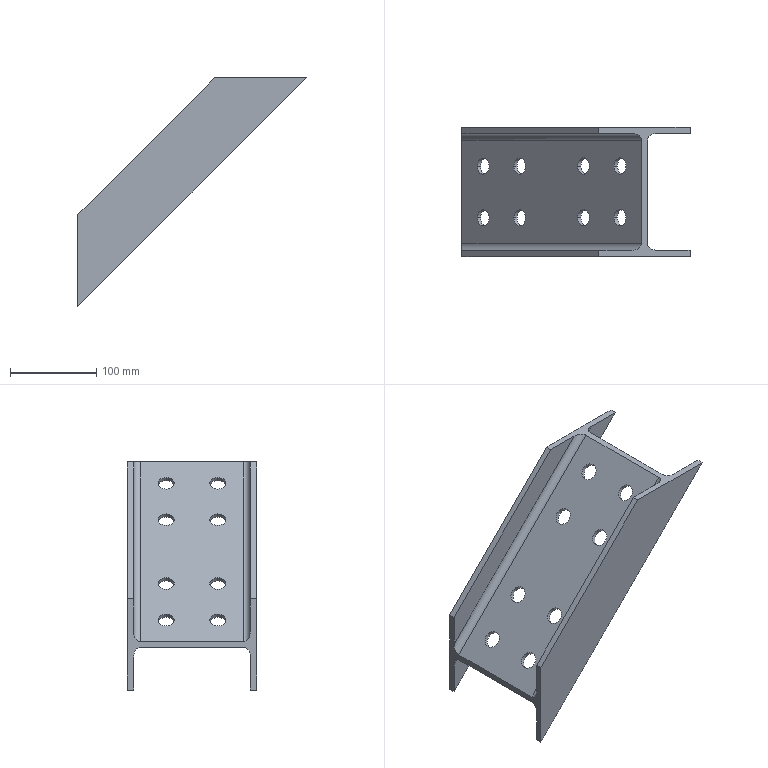Part | STEP file | 计量Diagonal Brace梁3_Default<As Machined> | 1 solid | 34 faces | box 265.165 x 150 x 265.165 mm | volume 524140 mm3 | cylinder 20 | plane 14 | commonest cylinder face diameters 19 x16 16 x4